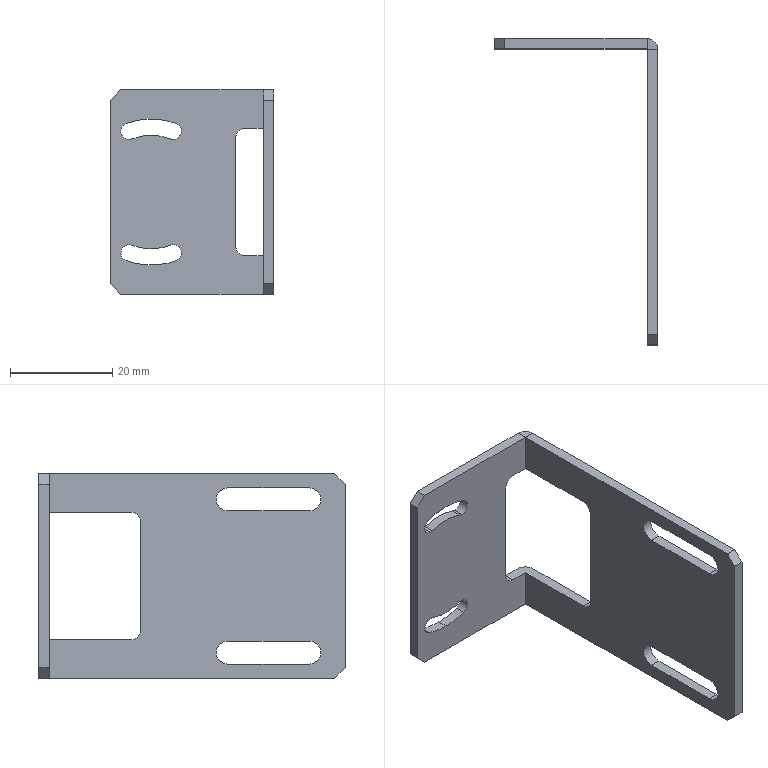Part | STEP file | 1 solid | 48 faces | box 32 x 60 x 40 mm | volume 5405 mm3 | cylinder 24 | plane 24 | commonest cylinder face diameters 3.2 x6 4 x4 4.5 x4 22.2 x3 28.6 x3 0.1 x2